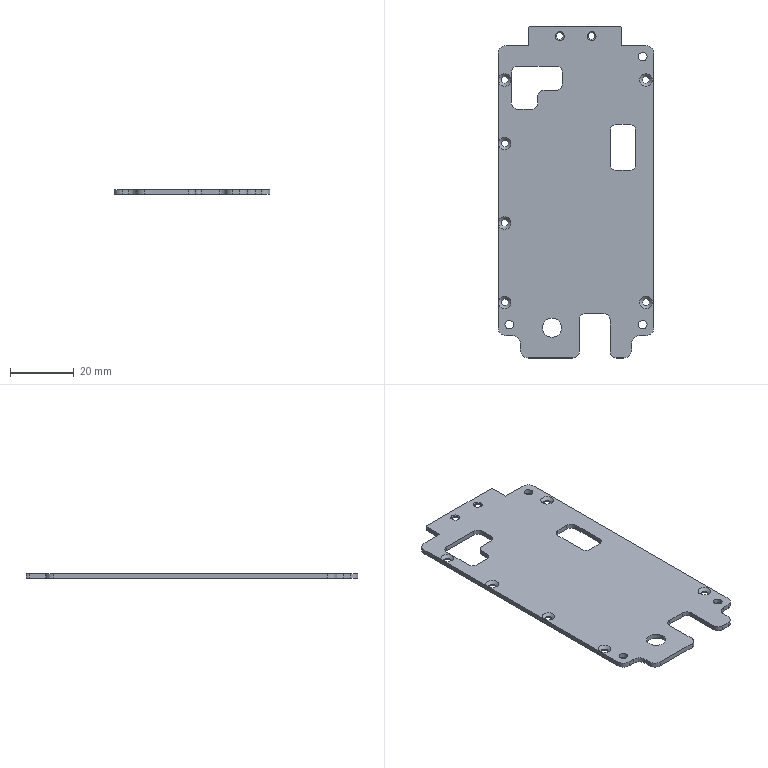Part | STEP file | Final stage amplifier cover 1 | 1 solid | 80 faces | box 49 x 104.5 x 1.5 mm | volume 6573 mm3 | cylinder 36 | plane 28 | cone 16 | commonest cylinder face diameters 4 x16 2.2 x8 5 x8 2.7 x3 6 x1